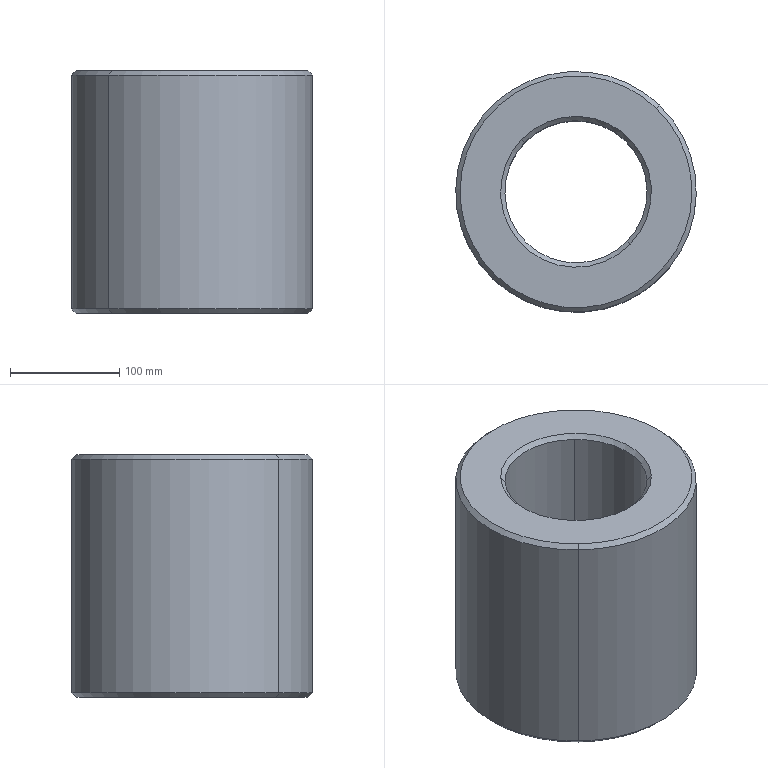Part | SolidWorks | features SplitBody 1 | 1 solid | 14 faces | box 220 x 220 x 222 mm | volume 5474696 mm3 | cone 8 | cylinder 4 | plane 2 | commonest cylinder face diameters 130 x2 220 x2
STEP:
#1=CARTESIAN_POINT('',(3039.854,334.056,1034.5));
#2=VERTEX_POINT('',#1);
#3=CARTESIAN_POINT('',(3192.146,492.824,1034.5));
#4=VERTEX_POINT('',#3);
#5=CARTESIAN_POINT('',(3116.,413.44,1034.5));
#6=DIRECTION('',(0.,0.,-1.));
#7=DIRECTION('',(-0.6922,-0.7217,0.));
#8=AXIS2_PLACEMENT_3D('',#5,#6,#7);
#9=CIRCLE('',#8,110.);
#10=EDGE_CURVE('',#2,#4,#9,.T.);
#11=ORIENTED_EDGE('',*,*,#10,.T.);
#12=CARTESIAN_POINT('',(3192.146,492.824,820.5));
#13=VERTEX_POINT('',#12);
#14=CARTESIAN_POINT('',(3192.146,492.824,1038.5));
#15=DIRECTION('',(0.,0.,-1.));
#16=VECTOR('',#15,1000.);
#17=LINE('',#14,#16);
#18=EDGE_CURVE('',#4,#13,#17,.T.);
#19=ORIENTED_EDGE('',*,*,#18,.T.);
#20=CARTESIAN_POINT('',(3039.854,334.056,820.5));
#21=VERTEX_POINT('',#20);
#22=CARTESIAN_POINT('',(3116.,413.44,820.5));
#23=DIRECTION('',(0.,0.,1.));
#24=DIRECTION('',(-0.6922,-0.7217,0.));
#25=AXIS2_PLACEMENT_3D('',#22,#23,#24);
#26=CIRCLE('',#25,110.);
#27=EDGE_CURVE('',#13,#21,#26,.T.);
#28=ORIENTED_EDGE('',*,*,#27,.T.);
#29=CARTESIAN_POINT('',(3039.854,334.056,1038.5));
#30=DIRECTION('',(0.,0.,-1.));
#31=VECTOR('',#30,1000.);
#32=LINE('',#29,#31);
#33=EDGE_CURVE('',#2,#21,#32,.T.);
#34=ORIENTED_EDGE('',*,*,#33,.F.);
#35=EDGE_LOOP('',(#11,#19,#28,#34));
#36=FACE_OUTER_BOUND('',#35,.T.);
#37=CARTESIAN_POINT('',(3116.,413.44,1038.5));
#38=DIRECTION('',(0.,0.,-1.));
#39=DIRECTION('',(-0.6922,-0.7217,0.));
#40=AXIS2_PLACEMENT_3D('',#37,#38,#39);
#41=CYLINDRICAL_SURFACE('',#40,110.);
#42=ADVANCED_FACE('',(#36),#41,.T.);
#43=CARTESIAN_POINT('',(3189.377,489.937,816.5));
#44=VERTEX_POINT('',#43);
#45=CARTESIAN_POINT('',(3042.623,336.943,816.5));
#46=VERTEX_POINT('',#45);
#47=CARTESIAN_POINT('',(3116.,413.44,816.5));
#48=DIRECTION('',(0.,0.,1.));
#49=DIRECTION('',(0.6922,0.7217,0.));
#50=AXIS2_PLACEMENT_3D('',#47,#48,#49);
#51=CIRCLE('',#50,106.);
#52=EDGE_CURVE('',#44,#46,#51,.T.);
#53=ORIENTED_EDGE('',*,*,#52,.T.);
#54=CARTESIAN_POINT('',(3039.854,334.056,820.5));
#55=DIRECTION('',(-0.4895,-0.5103,0.7071));
#56=VECTOR('',#55,1000.);
#57=LINE('',#54,#56);
#58=EDGE_CURVE('',#46,#21,#57,.T.);
#59=ORIENTED_EDGE('',*,*,#58,.T.);
#60=ORIENTED_EDGE('',*,*,#27,.F.);
#61=CARTESIAN_POINT('',(3192.146,492.824,820.5));
#62=DIRECTION('',(0.4895,0.5103,0.7071));
#63=VECTOR('',#62,1000.);
#64=LINE('',#61,#63);
#65=EDGE_CURVE('',#44,#13,#64,.T.);
#66=ORIENTED_EDGE('',*,*,#65,.F.);
#67=EDGE_LOOP('',(#53,#59,#60,#66));
#68=FACE_OUTER_BOUND('',#67,.T.);
#69=CARTESIAN_POINT('',(3116.,413.44,820.5));
#70=DIRECTION('',(0.,0.,1.));
#71=DIRECTION('',(0.6922,0.7217,0.));
#72=AXIS2_PLACEMENT_3D('',#69,#70,#71);
#73=CONICAL_SURFACE('',#72,110.,0.7854);
#74=ADVANCED_FACE('',(#68),#73,.T.);
#75=CARTESIAN_POINT('',(3042.623,336.943,1038.5));
#76=VERTEX_POINT('',#75);
#77=CARTESIAN_POINT('',(3189.377,489.937,1038.5));
#78=VERTEX_POINT('',#77);
#79=CARTESIAN_POINT('',(3116.,413.44,1038.5));
#80=DIRECTION('',(0.,0.,-1.));
#81=DIRECTION('',(-0.6922,-0.7217,0.));
#82=AXIS2_PLACEMENT_3D('',#79,#80,#81);
#83=CIRCLE('',#82,106.);
#84=EDGE_CURVE('',#76,#78,#83,.T.);
#85=ORIENTED_EDGE('',*,*,#84,.T.);
#86=CARTESIAN_POINT('',(3192.146,492.824,1034.5));
#87=DIRECTION('',(0.4895,0.5103,-0.7071));
#88=VECTOR('',#87,1000.);
#89=LINE('',#86,#88);
#90=EDGE_CURVE('',#78,#4,#89,.T.);
#91=ORIENTED_EDGE('',*,*,#90,.T.);
#92=ORIENTED_EDGE('',*,*,#10,.F.);
#93=CARTESIAN_POINT('',(3039.854,334.056,1034.5));
#94=DIRECTION('',(-0.4895,-0.5103,-0.7071));
#95=VECTOR('',#94,1000.);
#96=LINE('',#93,#95);
#97=EDGE_CURVE('',#76,#2,#96,.T.);
#98=ORIENTED_EDGE('',*,*,#97,.F.);
#99=EDGE_LOOP('',(#85,#91,#92,#98));
#100=FACE_OUTER_BOUND('',#99,.T.);
#101=CARTESIAN_POINT('',(3116.,413.44,1034.5));
#102=DIRECTION('',(0.,0.,-1.));
#103=DIRECTION('',(-0.6922,-0.7217,0.));
#104=AXIS2_PLACEMENT_3D('',#101,#102,#103);
#105=CONICAL_SURFACE('',#104,110.,0.7854);
#106=ADVANCED_FACE('',(#100),#105,.T.);
#107=CARTESIAN_POINT('',(3162.909,368.445,820.5));
#108=VERTEX_POINT('',#107);
#109=CARTESIAN_POINT('',(3071.005,366.532,820.5));
#110=VERTEX_POINT('',#109);
#111=CARTESIAN_POINT('',(3116.,413.44,820.5));
#112=DIRECTION('',(0.,0.,-1.));
#113=DIRECTION('',(-0.6922,-0.7217,0.));
#114=AXIS2_PLACEMENT_3D('',#111,#112,#113);
#115=CIRCLE('',#114,65.);
#116=EDGE_CURVE('',#108,#110,#115,.T.);
#117=ORIENTED_EDGE('',*,*,#116,.F.);
#118=CARTESIAN_POINT('',(3165.795,365.676,816.5));
#119=VERTEX_POINT('',#118);
#120=CARTESIAN_POINT('',(3165.795,365.676,816.5));
#121=DIRECTION('',(0.5103,-0.4895,-0.7071));
#122=VECTOR('',#121,1000.);
#123=LINE('',#120,#122);
#124=EDGE_CURVE('',#108,#119,#123,.T.);
#125=ORIENTED_EDGE('',*,*,#124,.T.);
#126=CARTESIAN_POINT('',(3066.205,461.204,816.5));
#127=VERTEX_POINT('',#126);
#128=CARTESIAN_POINT('',(3116.,413.44,816.5));
#129=DIRECTION('',(0.,0.,-1.));
#130=DIRECTION('',(-0.7217,0.6922,0.));
#131=AXIS2_PLACEMENT_3D('',#128,#129,#130);
#132=CIRCLE('',#131,69.);
#133=EDGE_CURVE('',#119,#127,#132,.T.);
#134=ORIENTED_EDGE('',*,*,#133,.T.);
#135=CARTESIAN_POINT('',(3069.091,458.436,820.5));
#136=VERTEX_POINT('',#135);
#137=CARTESIAN_POINT('',(3066.205,461.204,816.5));
#138=DIRECTION('',(-0.5103,0.4895,-0.7071));
#139=VECTOR('',#138,1000.);
#140=LINE('',#137,#139);
#141=EDGE_CURVE('',#136,#127,#140,.T.);
#142=ORIENTED_EDGE('',*,*,#141,.F.);
#143=CARTESIAN_POINT('',(3116.,413.44,820.5));
#144=DIRECTION('',(0.,0.,-1.));
#145=DIRECTION('',(-0.6922,-0.7217,0.));
#146=AXIS2_PLACEMENT_3D('',#143,#144,#145);
#147=CIRCLE('',#146,65.);
#148=EDGE_CURVE('',#110,#136,#147,.T.);
#149=ORIENTED_EDGE('',*,*,#148,.F.);
#150=EDGE_LOOP('',(#117,#125,#134,#142,#149));
#151=FACE_OUTER_BOUND('',#150,.T.);
#152=CARTESIAN_POINT('',(3116.,413.44,816.5));
#153=DIRECTION('',(0.,0.,-1.));
#154=DIRECTION('',(-0.7217,0.6922,0.));
#155=AXIS2_PLACEMENT_3D('',#152,#153,#154);
#156=CONICAL_SURFACE('',#155,69.,0.7854);
#157=ADVANCED_FACE('',(#151),#156,.F.);
#158=CARTESIAN_POINT('',(3069.091,458.436,1034.5));
#159=VERTEX_POINT('',#158);
#160=CARTESIAN_POINT('',(3071.005,366.532,1034.5));
#161=VERTEX_POINT('',#160);
#162=CARTESIAN_POINT('',(3116.,413.44,1034.5));
#163=DIRECTION('',(0.,0.,1.));
#164=DIRECTION('',(0.6922,0.7217,0.));
#165=AXIS2_PLACEMENT_3D('',#162,#163,#164);
#166=CIRCLE('',#165,65.);
#167=EDGE_CURVE('',#159,#161,#166,.T.);
#168=ORIENTED_EDGE('',*,*,#167,.F.);
#169=CARTESIAN_POINT('',(3066.205,461.204,1038.5));
#170=VERTEX_POINT('',#169);
#171=CARTESIAN_POINT('',(3066.205,461.204,1038.5));
#172=DIRECTION('',(-0.5103,0.4895,0.7071));
#173=VECTOR('',#172,1000.);
#174=LINE('',#171,#173);
#175=EDGE_CURVE('',#159,#170,#174,.T.);
#176=ORIENTED_EDGE('',*,*,#175,.T.);
#177=CARTESIAN_POINT('',(3165.795,365.676,1038.5));
#178=VERTEX_POINT('',#177);
#179=CARTESIAN_POINT('',(3116.,413.44,1038.5));
#180=DIRECTION('',(0.,0.,-1.));
#181=DIRECTION('',(0.7217,-0.6922,0.));
#182=AXIS2_PLACEMENT_3D('',#179,#180,#181);
#183=CIRCLE('',#182,69.);
#184=EDGE_CURVE('',#178,#170,#183,.T.);
#185=ORIENTED_EDGE('',*,*,#184,.F.);
#186=CARTESIAN_POINT('',(3162.909,368.445,1034.5));
#187=VERTEX_POINT('',#186);
#188=CARTESIAN_POINT('',(3165.795,365.676,1038.5));
#189=DIRECTION('',(0.5103,-0.4895,0.7071));
#190=VECTOR('',#189,1000.);
#191=LINE('',#188,#190);
#192=EDGE_CURVE('',#187,#178,#191,.T.);
#193=ORIENTED_EDGE('',*,*,#192,.F.);
#194=CARTESIAN_POINT('',(3116.,413.44,1034.5));
#195=DIRECTION('',(0.,0.,1.));
#196=DIRECTION('',(0.6922,0.7217,0.));
#197=AXIS2_PLACEMENT_3D('',#194,#195,#196);
#198=CIRCLE('',#197,65.);
#199=EDGE_CURVE('',#161,#187,#198,.T.);
#200=ORIENTED_EDGE('',*,*,#199,.F.);
#201=EDGE_LOOP('',(#168,#176,#185,#193,#200));
#202=FACE_OUTER_BOUND('',#201,.T.);
#203=CARTESIAN_POINT('',(3116.,413.44,1038.5));
#204=DIRECTION('',(0.,0.,1.));
#205=DIRECTION('',(0.7217,-0.6922,0.));
#206=AXIS2_PLACEMENT_3D('',#203,#204,#205);
#207=CONICAL_SURFACE('',#206,69.,0.7854);
#208=ADVANCED_FACE('',(#202),#207,.F.);
#209=ORIENTED_EDGE('',*,*,#199,.T.);
#210=CARTESIAN_POINT('',(3160.995,460.349,1034.5));
#211=VERTEX_POINT('',#210);
#212=CARTESIAN_POINT('',(3116.,413.44,1034.5));
#213=DIRECTION('',(0.,0.,1.));
#214=DIRECTION('',(0.6922,0.7217,0.));
#215=AXIS2_PLACEMENT_3D('',#212,#213,#214);
#216=CIRCLE('',#215,65.);
#217=EDGE_CURVE('',#187,#211,#216,.T.);
#218=ORIENTED_EDGE('',*,*,#217,.T.);
#219=CARTESIAN_POINT('',(3160.995,460.349,820.5));
#220=VERTEX_POINT('',#219);
#221=CARTESIAN_POINT('',(3160.995,460.349,1038.5));
#222=DIRECTION('',(0.,0.,-1.));
#223=VECTOR('',#222,1000.);
#224=LINE('',#221,#223);
#225=EDGE_CURVE('',#211,#220,#224,.T.);
#226=ORIENTED_EDGE('',*,*,#225,.T.);
#227=CARTESIAN_POINT('',(3116.,413.44,820.5));
#228=DIRECTION('',(0.,0.,-1.));
#229=DIRECTION('',(-0.6922,-0.7217,0.));
#230=AXIS2_PLACEMENT_3D('',#227,#228,#229);
#231=CIRCLE('',#230,65.);
#232=EDGE_CURVE('',#220,#108,#231,.T.);
#233=ORIENTED_EDGE('',*,*,#232,.T.);
#234=ORIENTED_EDGE('',*,*,#116,.T.);
#235=CARTESIAN_POINT('',(3071.005,366.532,1038.5));
#236=DIRECTION('',(0.,0.,-1.));
#237=VECTOR('',#236,1000.);
#238=LINE('',#235,#237);
#239=EDGE_CURVE('',#161,#110,#238,.T.);
#240=ORIENTED_EDGE('',*,*,#239,.F.);
#241=EDGE_LOOP('',(#209,#218,#226,#233,#234,#240));
#242=FACE_OUTER_BOUND('',#241,.T.);
#243=CARTESIAN_POINT('',(3116.,413.44,1038.5));
#244=DIRECTION('',(0.,0.,-1.));
#245=DIRECTION('',(-0.6922,-0.7217,0.));
#246=AXIS2_PLACEMENT_3D('',#243,#244,#245);
#247=CYLINDRICAL_SURFACE('',#246,65.);
#248=ADVANCED_FACE('',(#242),#247,.F.);
#249=ORIENTED_EDGE('',*,*,#18,.F.);
#250=CARTESIAN_POINT('',(3116.,413.44,1034.5));
#251=DIRECTION('',(0.,0.,-1.));
#252=DIRECTION('',(-0.6922,-0.7217,0.));
#253=AXIS2_PLACEMENT_3D('',#250,#251,#252);
#254=CIRCLE('',#253,110.);
#255=EDGE_CURVE('',#4,#2,#254,.T.);
#256=ORIENTED_EDGE('',*,*,#255,.T.);
#257=ORIENTED_EDGE('',*,*,#33,.T.);
#258=CARTESIAN_POINT('',(3116.,413.44,820.5));
#259=DIRECTION('',(0.,0.,1.));
#260=DIRECTION('',(-0.6922,-0.7217,0.));
#261=AXIS2_PLACEMENT_3D('',#258,#259,#260);
#262=CIRCLE('',#261,110.);
#263=EDGE_CURVE('',#21,#13,#262,.T.);
#264=ORIENTED_EDGE('',*,*,#263,.T.);
#265=EDGE_LOOP('',(#249,#256,#257,#264));
#266=FACE_OUTER_BOUND('',#265,.T.);
#267=CARTESIAN_POINT('',(3116.,413.44,1038.5));
#268=DIRECTION('',(0.,0.,-1.));
#269=DIRECTION('',(-0.6922,-0.7217,0.));
#270=AXIS2_PLACEMENT_3D('',#267,#268,#269);
#271=CYLINDRICAL_SURFACE('',#270,110.);
#272=ADVANCED_FACE('',(#266),#271,.T.);
#273=ORIENTED_EDGE('',*,*,#58,.F.);
#274=CARTESIAN_POINT('',(3116.,413.44,816.5));
#275=DIRECTION('',(0.,0.,1.));
#276=DIRECTION('',(0.6922,0.7217,0.));
#277=AXIS2_PLACEMENT_3D('',#274,#275,#276);
#278=CIRCLE('',#277,106.);
#279=EDGE_CURVE('',#46,#44,#278,.T.);
#280=ORIENTED_EDGE('',*,*,#279,.T.);
#281=ORIENTED_EDGE('',*,*,#65,.T.);
#282=ORIENTED_EDGE('',*,*,#263,.F.);
#283=EDGE_LOOP('',(#273,#280,#281,#282));
#284=FACE_OUTER_BOUND('',#283,.T.);
#285=CARTESIAN_POINT('',(3116.,413.44,820.5));
#286=DIRECTION('',(0.,0.,1.));
#287=DIRECTION('',(0.6922,0.7217,0.));
#288=AXIS2_PLACEMENT_3D('',#285,#286,#287);
#289=CONICAL_SURFACE('',#288,110.,0.7854);
#290=ADVANCED_FACE('',(#284),#289,.T.);
#291=ORIENTED_EDGE('',*,*,#90,.F.);
#292=CARTESIAN_POINT('',(3116.,413.44,1038.5));
#293=DIRECTION('',(0.,0.,-1.));
#294=DIRECTION('',(-0.6922,-0.7217,0.));
#295=AXIS2_PLACEMENT_3D('',#292,#293,#294);
#296=CIRCLE('',#295,106.);
#297=EDGE_CURVE('',#78,#76,#296,.T.);
#298=ORIENTED_EDGE('',*,*,#297,.T.);
#299=ORIENTED_EDGE('',*,*,#97,.T.);
#300=ORIENTED_EDGE('',*,*,#255,.F.);
#301=EDGE_LOOP('',(#291,#298,#299,#300));
#302=FACE_OUTER_BOUND('',#301,.T.);
#303=CARTESIAN_POINT('',(3116.,413.44,1034.5));
#304=DIRECTION('',(0.,0.,-1.));
#305=DIRECTION('',(-0.6922,-0.7217,0.));
#306=AXIS2_PLACEMENT_3D('',#303,#304,#305);
#307=CONICAL_SURFACE('',#306,110.,0.7854);
#308=ADVANCED_FACE('',(#302),#307,.T.);
#309=CARTESIAN_POINT('',(3116.,413.44,816.5));
#310=DIRECTION('',(0.,0.,-1.));
#311=DIRECTION('',(-0.7217,0.6922,0.));
#312=AXIS2_PLACEMENT_3D('',#309,#310,#311);
#313=CIRCLE('',#312,69.);
#314=EDGE_CURVE('',#127,#119,#313,.T.);
#315=ORIENTED_EDGE('',*,*,#314,.F.);
#316=ORIENTED_EDGE('',*,*,#133,.F.);
#317=EDGE_LOOP('',(#315,#316));
#318=FACE_BOUND('',#317,.T.);
#319=ORIENTED_EDGE('',*,*,#52,.F.);
#320=ORIENTED_EDGE('',*,*,#279,.F.);
#321=EDGE_LOOP('',(#319,#320));
#322=FACE_OUTER_BOUND('',#321,.T.);
#323=CARTESIAN_POINT('',(3116.,413.44,816.5));
#324=DIRECTION('',(0.,0.,1.));
#325=DIRECTION('',(0.6922,0.7217,0.));
#326=AXIS2_PLACEMENT_3D('',#323,#324,#325);
#327=PLANE('',#326);
#328=ADVANCED_FACE('',(#318,#322),#327,.F.);
#329=ORIENTED_EDGE('',*,*,#184,.T.);
#330=CARTESIAN_POINT('',(3116.,413.44,1038.5));
#331=DIRECTION('',(0.,0.,-1.));
#332=DIRECTION('',(0.7217,-0.6922,0.));
#333=AXIS2_PLACEMENT_3D('',#330,#331,#332);
#334=CIRCLE('',#333,69.);
#335=EDGE_CURVE('',#170,#178,#334,.T.);
#336=ORIENTED_EDGE('',*,*,#335,.T.);
#337=EDGE_LOOP('',(#329,#336));
#338=FACE_BOUND('',#337,.T.);
#339=ORIENTED_EDGE('',*,*,#84,.F.);
#340=ORIENTED_EDGE('',*,*,#297,.F.);
#341=EDGE_LOOP('',(#339,#340));
#342=FACE_OUTER_BOUND('',#341,.T.);
#343=CARTESIAN_POINT('',(3116.,413.44,1038.5));
#344=DIRECTION('',(0.,0.,1.));
#345=DIRECTION('',(0.6922,0.7217,0.));
#346=AXIS2_PLACEMENT_3D('',#343,#344,#345);
#347=PLANE('',#346);
#348=ADVANCED_FACE('',(#338,#342),#347,.T.);
#349=ORIENTED_EDGE('',*,*,#124,.F.);
#350=ORIENTED_EDGE('',*,*,#232,.F.);
#351=CARTESIAN_POINT('',(3116.,413.44,820.5));
#352=DIRECTION('',(0.,0.,-1.));
#353=DIRECTION('',(-0.6922,-0.7217,0.));
#354=AXIS2_PLACEMENT_3D('',#351,#352,#353);
#355=CIRCLE('',#354,65.);
#356=EDGE_CURVE('',#136,#220,#355,.T.);
#357=ORIENTED_EDGE('',*,*,#356,.F.);
#358=ORIENTED_EDGE('',*,*,#141,.T.);
#359=ORIENTED_EDGE('',*,*,#314,.T.);
#360=EDGE_LOOP('',(#349,#350,#357,#358,#359));
#361=FACE_OUTER_BOUND('',#360,.T.);
#362=CARTESIAN_POINT('',(3116.,413.44,816.5));
#363=DIRECTION('',(0.,0.,-1.));
#364=DIRECTION('',(-0.7217,0.6922,0.));
#365=AXIS2_PLACEMENT_3D('',#362,#363,#364);
#366=CONICAL_SURFACE('',#365,69.,0.7854);
#367=ADVANCED_FACE('',(#361),#366,.F.);
#368=ORIENTED_EDGE('',*,*,#175,.F.);
#369=CARTESIAN_POINT('',(3116.,413.44,1034.5));
#370=DIRECTION('',(0.,0.,1.));
#371=DIRECTION('',(0.6922,0.7217,0.));
#372=AXIS2_PLACEMENT_3D('',#369,#370,#371);
#373=CIRCLE('',#372,65.);
#374=EDGE_CURVE('',#211,#159,#373,.T.);
#375=ORIENTED_EDGE('',*,*,#374,.F.);
#376=ORIENTED_EDGE('',*,*,#217,.F.);
#377=ORIENTED_EDGE('',*,*,#192,.T.);
#378=ORIENTED_EDGE('',*,*,#335,.F.);
#379=EDGE_LOOP('',(#368,#375,#376,#377,#378));
#380=FACE_OUTER_BOUND('',#379,.T.);
#381=CARTESIAN_POINT('',(3116.,413.44,1038.5));
#382=DIRECTION('',(0.,0.,1.));
#383=DIRECTION('',(0.7217,-0.6922,0.));
#384=AXIS2_PLACEMENT_3D('',#381,#382,#383);
#385=CONICAL_SURFACE('',#384,69.,0.7854);
#386=ADVANCED_FACE('',(#380),#385,.F.);
#387=ORIENTED_EDGE('',*,*,#225,.F.);
#388=ORIENTED_EDGE('',*,*,#374,.T.);
#389=ORIENTED_EDGE('',*,*,#167,.T.);
#390=ORIENTED_EDGE('',*,*,#239,.T.);
#391=ORIENTED_EDGE('',*,*,#148,.T.);
#392=ORIENTED_EDGE('',*,*,#356,.T.);
#393=EDGE_LOOP('',(#387,#388,#389,#390,#391,#392));
#394=FACE_OUTER_BOUND('',#393,.T.);
#395=CARTESIAN_POINT('',(3116.,413.44,1038.5));
#396=DIRECTION('',(0.,0.,-1.));
#397=DIRECTION('',(-0.6922,-0.7217,0.));
#398=AXIS2_PLACEMENT_3D('',#395,#396,#397);
#399=CYLINDRICAL_SURFACE('',#398,65.);
#400=ADVANCED_FACE('',(#394),#399,.F.);
#401=CLOSED_SHELL('',(#42,#74,#106,#157,#208,#248,#272,#290,#308,#328,#348,#367,#386,#400));
#402=MANIFOLD_SOLID_BREP('',#401);
#403=CARTESIAN_POINT('',(0.,0.,0.));
#404=DIRECTION('',(0.,0.,1.));
#405=DIRECTION('',(1.,0.,0.));
#406=AXIS2_PLACEMENT_3D('',#403,#404,#405);
#407=(LENGTH_UNIT()NAMED_UNIT(*)SI_UNIT(.MILLI.,.METRE.));
#408=UNCERTAINTY_MEASURE_WITH_UNIT(LENGTH_MEASURE(0.00001),#407,'','');
#409=(NAMED_UNIT(*)PLANE_ANGLE_UNIT()SI_UNIT($,.RADIAN.));
#410=(NAMED_UNIT(*)SI_UNIT($,.STERADIAN.)SOLID_ANGLE_UNIT());
#411=(GEOMETRIC_REPRESENTATION_CONTEXT(3)GLOBAL_UNCERTAINTY_ASSIGNED_CONTEXT((#408))GLOBAL_UNIT_ASSIGNED_CONTEXT((#407,#409,#410))REPRESENTATION_CONTEXT('',''));
#412=ADVANCED_BREP_SHAPE_REPRESENTATION('',(#402,#406),#411);